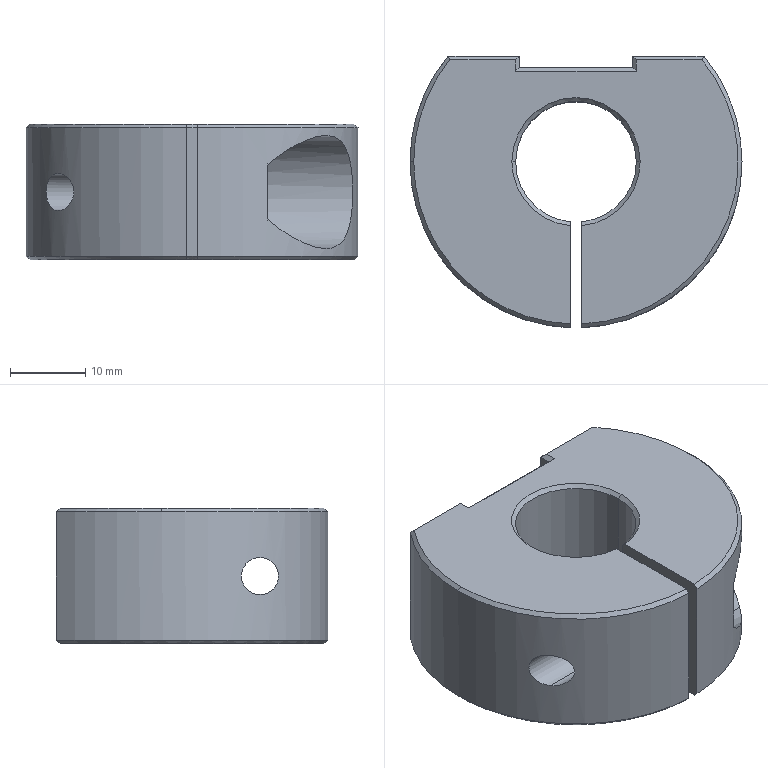Part | SolidWorks | features BaseBody 1 | 1 solid | 59 faces | box 44 x 35.987 x 18 mm | volume 17414 mm3 | cone 22 | plane 20 | cylinder 17 | commonest cylinder face diameters 4.134 x4 15 x3 16 x3 44 x3 4.917 x2 6.6 x2